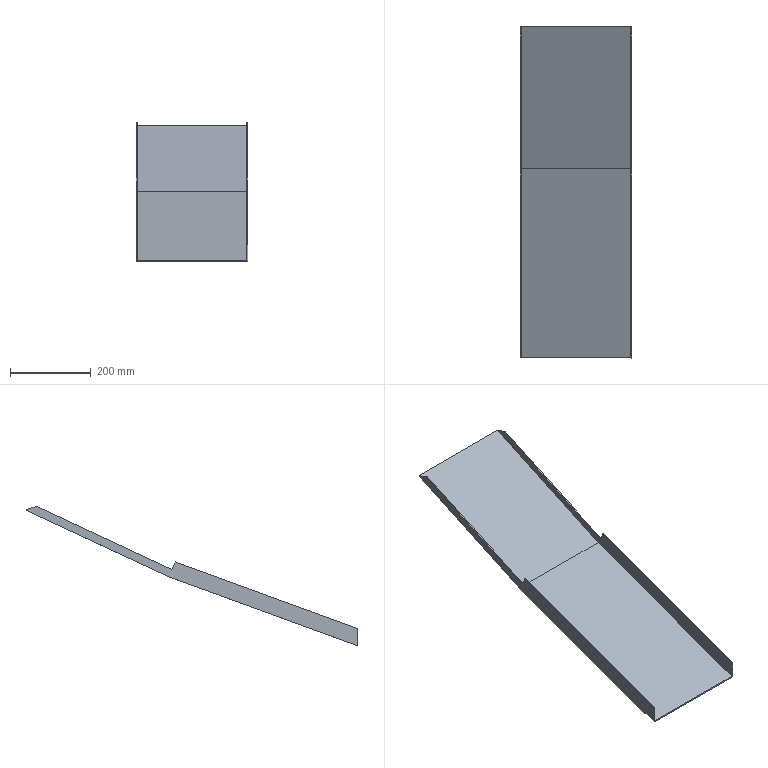Part | NX | features solid 2 | 1 solid | 31 faces | box 275.083 x 820.571 x 345.137 mm | volume 589442 mm3 | plane 29 | cylinder 2 | commonest cylinder face diameters 40 x2